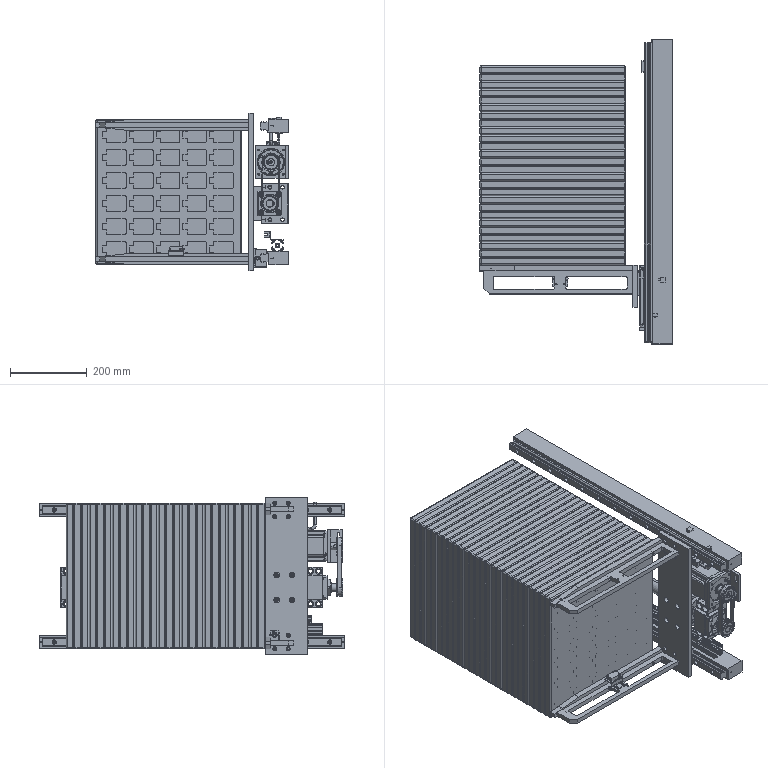Part | SolidWorks | features ReferencePattern 31, LocalLPattern 3, AEMSimFeature 1, CompositeCurve 1 | 110 solids | 20559 faces | volume 52361589 mm3 | cylinder 9761 | plane 8322 | torus 1568 | spline 363 | cone 337 | sphere 208 | commonest cylinder face diameters 6 x8180 1.1 x132 0.5 x131 6.55 x116 9 x108 5 x92